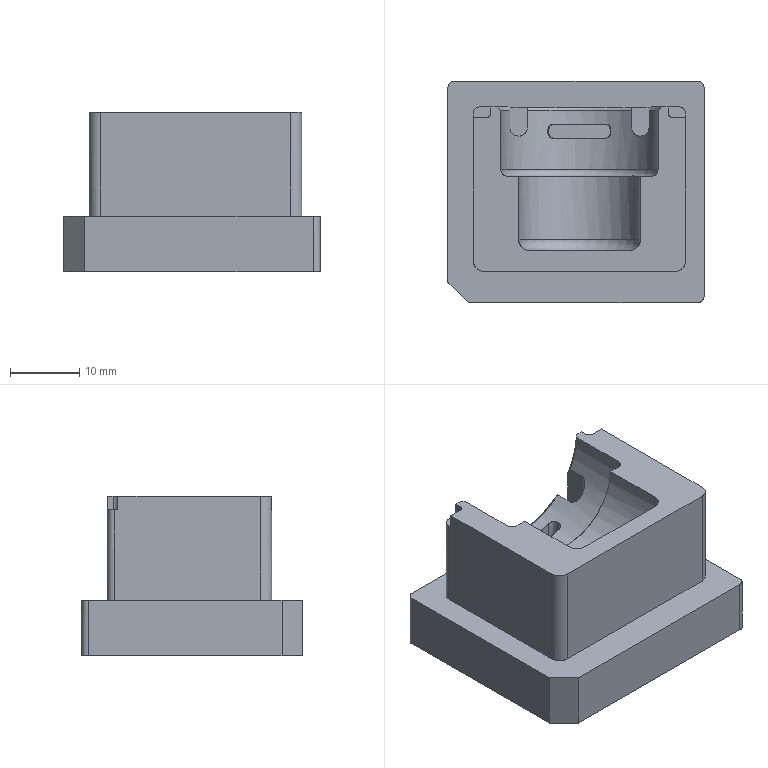NC program | PowerMill | posted with a generic post | part box 37 x 32 x 23 mm
Lines 26967 to 27634 of 159067:
N27064 M6
N27065 S8500 M03
N27066 G00 G90 X0.0 Y0.0
N27067 G43 Z11.8 H3
N27068
N27069 G05 P10000 R8
N27070 X-12.7401 Y22.8793
N27071 Z-1.156
N27072 G01 Z-2.356 F360.0
N27073 X-12.7403 Y17.6043 F600.0
N27074 X-12.8666 Y17.4744
N27075 G00 Z2.8538
N27076 G01 X-25.4619 Y11.9052 F10000.0
N27077 G00 Z-1.156
N27078 G01 Z-2.356 F360.0
N27079 X-20.1929 Y11.6533 F600.0
N27080 G03 X-19.9391 Y12.0208 I-0.3314 J0.5002
N27081 G01 X-19.8095 Y12.4495
N27082 X-19.6538 Y12.8389
N27083 X-19.4987 Y13.1574
N27084 X-19.3232 Y13.4633
N27085 X-19.2241 Y13.6177
N27086 X-18.9592 Y13.9792
N27087 X-18.6419 Y14.3407
N27088 X-18.5304 Y14.4536
N27089 X-18.134 Y14.804
N27090 X-17.7375 Y15.091
N27091 X-17.6051 Y15.1755
N27092 X-17.2749 Y15.3622
N27093 X-16.9447 Y15.5192
N27094 X-16.2702 Y15.7923
N27095 G03 X-16.0633 Y15.9321 I-0.2251 J0.5562
N27096 G01 X-15.7004 Y16.2688
N27097 X-15.359 Y16.5339
N27098 X-15.0563 Y16.7332
N27099 X-14.8146 Y16.8723
N27100 X-14.5661 Y16.9986
N27101 X-14.1697 Y17.1669
N27102 X-13.7733 Y17.299
N27103 X-13.3769 Y17.3969
N27104 X-12.9115 Y17.4687
N27105 G03 X-12.582 Y17.6043 I-0.0533 J0.5977
N27106 G00 Z2.8538
N27107 G01 X13.525 Y22.879 F10000.0
N27108 G00 Z-1.156
N27109 G01 Z-2.356 F360.0
N27110 X13.5779 Y17.6043 F600.0
N27111 G03 X13.9074 Y17.4687 I0.3828 J0.4621
N27112 G01 X14.3728 Y17.3969
N27113 X14.6204 Y17.3371
N27114 X14.8653 Y17.267
N27115 X15.1656 Y17.1669
N27116 X15.562 Y16.9986
N27117 X15.8105 Y16.8723
N27118 X16.0521 Y16.7332
N27119 X16.3549 Y16.5339
N27120 X16.6959 Y16.2694
N27121 X17.0591 Y15.9321
N27122 G03 X17.266 Y15.7923 I0.4321 J0.4164
N27123 G01 X17.9406 Y15.5192
N27124 X18.2704 Y15.3622
N27125 X18.601 Y15.1755
N27126 X18.7334 Y15.091
N27127 X19.1298 Y14.804
N27128 X19.5835 Y14.3966
N27129 X19.9014 Y14.0454
N27130 X20.22 Y13.6177
N27131 X20.3191 Y13.4633
N27132 X20.4947 Y13.1574
N27133 X20.6472 Y12.8453
N27134 X20.8047 Y12.4495
N27135 X20.9261 Y12.06
N27136 X21.0148 Y11.6706
N27137 X21.0771 Y11.219
N27138 G03 X21.2043 Y10.8918 I0.5983 J0.0443
N27139 G00 Z4.0
N27140 G01 X-24.9518 Y-13.4611 F10000.0
N27141 G00 Z0.8
N27142 G01 Z-0.4 F360.0
N27143 X-19.9022 Y-11.9356 F600.0
N27144 X20.9006 Y-11.9252
N27145 X21.042 Y-11.3912
N27146 X21.1226 Y-10.9631
N27147 X21.177 Y-10.5097
N27148 X21.2021 Y-10.0577
N27149 X21.2041 Y-7.0021
N27150 X-20.2078 Y-7.0126
N27151 X-20.208 Y-2.0896
N27152 X-2.9417 Y-2.0852
N27153 X-2.9457 Y2.3697
N27154 X-2.9685 Y2.7272
N27155 X-2.9834 Y2.8378
N27156 X-20.2082 Y2.8334
N27157 X-20.2084 Y7.7564
N27158 X-5.5055 Y7.7602
N27159 X-5.5061 Y11.8451
N27160 G03 X-5.589 Y12.6832 I-5.7385 J-0.1442
N27161 G01 X-19.8266 Y12.6796
N27162 G00 Z4.0
N27163 G01 X-1.3376 Y-2.083 F10000.0
N27164 G00 Z0.8
N27165 G01 Z-0.4 F360.0
N27166 X3.9374 Y-2.0835 F600.0
N27167 X21.204 Y-2.0791
N27168 X21.2038 Y2.8439
N27169 X3.9772 Y2.8395
N27170 G02 X4.2203 Y3.9177 I5.4024 J-0.6514
N27171 G01 X4.3607 Y4.2897
N27172 X4.5799 Y4.745
N27173 X4.6454 Y4.8536
N27174 G02 X5.1997 Y5.6551 I4.3119 J-2.3898
N27175 G01 X5.4158 Y5.8958
N27176 X5.7046 Y6.1763
N27177 X5.9771 Y6.4062
N27178 X6.2349 Y6.5958
N27179 X6.5011 Y6.7732
N27180 X6.5014 Y7.7632
N27181 X21.2037 Y7.7669
N27182 X21.2006 Y10.8927
N27183 G03 X21.0747 Y11.8712 I-5.6314 J-0.227
N27184 G03 X20.8204 Y12.6898 I-5.3043 J-1.199
N27185 G01 X6.5867 Y12.6862
N27186 G00 Z11.8
N27187 G05 P0
N27188 (---------------)
N27189 ( END TOOLPATH : 粗公基准台01-平坦面平行-D10 )
N27190 (---------------)
N27191 ( START TOOLPATH : 粗公基准台01-基准面偏置-D10 )
N27192 (---------------)
N27193 G00 X0.0 Y0.0 Z9.8
N27194 G05 P10000 R8
N27195 X-8.4072 Y-26.625
N27196 Z-14.0
N27197 G01 Z-15.2 F360.0
N27198 Y-21.35 F600.0
N27199 X0.7919 Y-16.7504
N27200 X-13.4626 Y-16.7466
N27201 X-13.8585 Y-16.7231
N27202 X-14.2545 Y-16.6774
N27203 X-15.0464 Y-16.5113
N27204 X-15.4424 Y-16.3928
N27205 X-15.8383 Y-16.2445
N27206 X-16.2343 Y-16.0695
N27207 X-16.6303 Y-15.8609
N27208 X-17.1233 Y-15.556
N27209 X-17.4222 Y-15.3388
N27210 X-17.8769 Y-14.959
N27211 X-18.2141 Y-14.6284
N27212 X-18.4232 Y-14.4
N27213 X-18.6258 Y-14.1528
N27214 X-18.8201 Y-13.8991
N27215 X-19.006 Y-13.6265
N27216 X-19.1529 Y-13.3844
N27217 X-19.372 Y-12.9907
N27218 X-19.5528 Y-12.597
N27219 X-19.6866 Y-12.2684
N27220 X-19.8366 Y-11.8097
N27221 X-19.9393 Y-11.4161
N27222 X-20.016 Y-11.0224
N27223 X-20.07 Y-10.6288
N27224 X-20.0988 Y-10.2351
N27225 X-20.1088 Y-9.4478
N27226 X-20.1061 Y11.4161
N27227 X-20.0825 Y11.8097
N27228 X-20.0454 Y12.1426
N27229 X-19.9627 Y12.597
N27230 X-19.7979 Y13.1998
N27231 X-19.7337 Y13.3844
N27232 X-19.5764 Y13.778
N27233 X-19.3857 Y14.1717
N27234 X-19.207 Y14.4858
N27235 X-19.006 Y14.7998
N27236 X-18.8923 Y14.959
N27237 X-18.578 Y15.348
N27238 X-18.2048 Y15.7463
N27239 X-17.8135 Y16.091
N27240 X-17.4222 Y16.3891
N27241 X-17.2041 Y16.5336
N27242 X-16.6303 Y16.8565
N27243 X-16.2343 Y17.0358
N27244 X-15.8383 Y17.1825
N27245 X-15.3573 Y17.3209
N27246 X-15.0464 Y17.3909
N27247 X-14.6505 Y17.454
N27248 X-14.2545 Y17.4901
N27249 X-13.5751 Y17.5049
N27250 X15.0464 Y17.5016
N27251 X15.4424 Y17.4753
N27252 X15.8383 Y17.427
N27253 X16.3534 Y17.3209
N27254 X16.6303 Y17.2471
N27255 X17.0262 Y17.115
N27256 X17.4222 Y16.9526
N27257 X17.8081 Y16.762
N27258 X18.2141 Y16.5252
N27259 X18.6101 Y16.2502
N27260 X19.006 Y15.9239
N27261 X19.2001 Y15.7463
N27262 X19.5204 Y15.4103
N27263 X19.8884 Y14.959
N27264 X20.1552 Y14.5653
N27265 X20.3818 Y14.1717
N27266 X20.5898 Y13.738
N27267 X20.7298 Y13.3844
N27268 X20.8314 Y13.0824
N27269 X20.9587 Y12.597
N27270 X21.0325 Y12.2034
N27271 X21.0778 Y11.8097
N27272 X21.1024 Y11.4161
N27273 X21.1049 Y-9.4478
N27274 X21.0941 Y-10.2351
N27275 X21.0657 Y-10.6288
N27276 X21.0121 Y-11.0224
N27277 X20.9352 Y-11.4161
N27278 X20.8319 Y-11.8097
N27279 X20.7228 Y-12.1549
N27280 X20.5481 Y-12.597
N27281 X20.3679 Y-12.9907
N27282 X20.149 Y-13.3844
N27283 X19.9842 Y-13.6542
N27284 X19.7979 Y-13.9241
N27285 X19.6069 Y-14.1717
N27286 X19.3279 Y-14.5027
N27287 X19.006 Y-14.8337
N27288 X18.873 Y-14.959
N27289 X18.5435 Y-15.2389
N27290 X18.2141 Y-15.4895
N27291 X17.8205 Y-15.7463
N27292 X17.4222 Y-15.9739
N27293 X17.0262 Y-16.1614
N27294 X16.6303 Y-16.3253
N27295 X15.9605 Y-16.5336
N27296 X15.4424 Y-16.6461
N27297 X15.0464 Y-16.7043
N27298 X14.2545 Y-16.7504
N27299 X0.7919
N27300 G00 Z9.8
N27301 G05 P0
N27302 (---------------)
N27303 ( END TOOLPATH : 粗公基准台01-基准面偏置-D10 )
N27304 (---------------)
N27305 ( START TOOLPATH : 粗公基准台01-外形侧光-D10 )
N27306 (---------------)
N27307 G00 X0.0 Y0.0 Z10.8
N27308 G05 P10000 R8
N27309 X19.6602 Y-14.3443
N27310 Z-13.97
N27311 G01 Z-15.17 F360.0
N27312 G03 X18.5771 Y-14.7249 I-0.0821 J-1.4977 F600.0
N27313 G02 X14.1984 Y-16.38 I-4.3278 J4.8298
N27314 G01 X-13.1666
N27315 G02 X-19.7384 Y-9.9389 I-0.0854 J6.486
N27316 G01 X-19.7386 Y11.2314
N27317 G02 X-13.9402 Y17.1338 I5.8849 J0.0182
N27318 G01 X0.5163 Y17.1342
N27319 X14.7151 Y17.1345
N27320 G02 X20.7344 Y11.2296 I0.1299 J-5.888
N27321 G01 X20.7343 Y-9.9404
N27322 G02 X19.792 Y-13.2619 I-6.485 J0.0453
N27323 G02 X18.5771 Y-14.7249 I-5.5426 J3.3668
N27324 G03 X18.0804 Y-15.7599 I1.001 J-1.1171
N27325 G01 X19.5989 Y-14.2944
N27326 G03 X18.5151 Y-14.6731 I-0.0848 J-1.4976
N27327 G02 X14.1984 Y-16.3 I-4.2656 J4.7779
N27328 G01 X-13.1658
N27329 G02 X-19.6584 Y-9.9389 I-0.0862 J6.406
N27330 G01 X-19.6586 Y11.2296
N27331 G02 X-13.9402 Y17.0538 I5.8049 J0.02
N27332 G01 X0.5163 Y17.0545
N27333 X14.7147
N27334 G02 X20.6544 Y11.2296 I0.1304 J-5.8079
N27335 G01 X20.6543 Y-9.9389
N27336 G02 X19.7236 Y-13.2204 I-6.4049 J0.0437
N27337 G02 X18.5151 Y-14.6731 I-5.4742 J3.3252
N27338 G03 X18.0165 Y-15.7072 I0.999 J-1.1189
N27339 G00 Z10.8
N27340 G05 P0
N27341 (---------------)
N27342 ( END TOOLPATH : 粗公基准台01-外形侧光-D10 )
N27343 (---------------)
N27344 ( START TOOLPATH : 粗公基准台01-基准台侧光-D10 )
N27345 (---------------)
N27346 G00 X0.0 Y0.0 Z9.8
N27347 G05 P10000 R8
N27348 X23.9377 Y-24.0084
N27349 Z-21.9
N27350 G01 Z-23.1 F360.0
N27351 G03 X20.9814 Y-19.976 I-1.4782 J2.0162 F600.0
N27352 G01 X20.8321 Y-20.0854
N27353 X20.8289 Y-20.0877
N27354 X20.8256 Y-20.0898
N27355 X20.3786 Y-20.3545
N27356 X20.3757 Y-20.3561
N27357 X20.3728 Y-20.3576
N27358 X19.9258 Y-20.5748
N27359 X19.9239 Y-20.5758
N27360 X19.9219 Y-20.5766
N27361 X19.783 Y-20.6351
N27362 X19.7814 Y-20.6357
N27363 X19.7798 Y-20.6363
N27364 X19.4717 Y-20.7508
N27365 X19.4692 Y-20.7517
N27366 X19.4667 Y-20.7525
N27367 X19.0197 Y-20.8857
N27368 X19.0169 Y-20.8864
N27369 X19.0141 Y-20.8871
N27370 X18.5671 Y-20.9854
N27371 X18.5639 Y-20.986
N27372 X18.5608 Y-20.9865
N27373 X18.1138 Y-21.0477
N27374 X18.111 Y-21.0481
N27375 X18.1081 Y-21.0483
N27376 X17.6611 Y-21.0774
N27377 X17.6588 Y-21.0775
N27378 X17.6564 Y-21.0776
N27379 X17.2094 Y-21.08
N27380 X17.2092
N27381 X17.2089
N27382 X-15.421
N27383 X-15.4222
N27384 X-15.4234
N27385 X-15.8704 Y-21.0664
N27386 X-15.8739 Y-21.0663
N27387 X-15.8775 Y-21.0659
N27388 X-16.3244 Y-21.0126
N27389 X-16.328 Y-21.0121
N27390 X-16.3316 Y-21.0114
N27391 X-16.7786 Y-20.9164
N27392 X-16.7822 Y-20.9156
N27393 X-16.7858 Y-20.9145
N27394 X-17.2327 Y-20.7753
N27395 X-17.2364 Y-20.774
N27396 X-17.2399 Y-20.7727
N27397 X-17.6869 Y-20.5851
N27398 X-17.6905 Y-20.5835
N27399 X-17.6941 Y-20.5817
N27400 X-18.141 Y-20.3394
N27401 X-18.1438 Y-20.3379
N27402 X-18.1465 Y-20.3362
N27403 X-18.3848 Y-20.1814
N27404 X-18.3866 Y-20.1802
N27405 X-18.3883 Y-20.179
N27406 X-18.5971 Y-20.0267
N27407 X-18.5993 Y-20.025
N27408 X-18.6015 Y-20.0232
N27409 X-18.9502 Y-19.7285
N27410 X-18.952 Y-19.7269
N27411 X-18.9538 Y-19.7253
N27412 X-19.052 Y-19.6317
N27413 X-19.0528 Y-19.6311
N27414 X-19.0535 Y-19.6304
N27415 X-22.0892 Y-16.595
N27416 X-22.0895 Y-16.5947
N27417 X-22.0899 Y-16.5943
N27418 X-22.1831 Y-16.4988
N27419 X-22.1847 Y-16.4971
N27420 X-22.1863 Y-16.4953
N27421 X-22.4902 Y-16.1438
N27422 X-22.4921 Y-16.1417
N27423 X-22.4938 Y-16.1394
N27424 X-22.6368 Y-15.9484
N27425 X-22.6381 Y-15.9466
N27426 X-22.6393 Y-15.9448
N27427 X-22.81 Y-15.6889
N27428 X-22.8118 Y-15.6861
N27429 X-22.8134 Y-15.6833
N27430 X-23.0612 Y-15.2363
N27431 X-23.063 Y-15.2328
N27432 X-23.0647 Y-15.2291
N27433 X-23.257 Y-14.7821
N27434 X-23.2585 Y-14.7786
N27435 X-23.2597 Y-14.775
N27436 X-23.4033 Y-14.328
N27437 X-23.4043 Y-14.3244
N27438 X-23.4052 Y-14.3208
N27439 X-23.5042 Y-13.8739
N27440 X-23.5049 Y-13.8703
N27441 X-23.5055 Y-13.8667
N27442 X-23.5626 Y-13.4197
N27443 X-23.563 Y-13.4161
N27444 X-23.5632 Y-13.4126
N27445 X-23.58 Y-12.9656
N27446 Y-12.9641
N27447 Y-12.9626
N27448 Y14.7505
N27449 Y14.7509
N27450 Y14.7512
N27451 X-23.5761 Y15.1982
N27452 X-23.576 Y15.2007
N27453 X-23.5759 Y15.2032
N27454 X-23.5442 Y15.6501
N27455 X-23.544 Y15.6531
N27456 X-23.5436 Y15.6559
N27457 X-23.479 Y16.1029
N27458 X-23.4785 Y16.1061
N27459 X-23.4778 Y16.1092
N27460 X-23.3765 Y16.5562
N27461 X-23.3758 Y16.5591
N27462 X-23.375 Y16.562
N27463 X-23.2375 Y17.009
N27464 X-23.2366 Y17.0116
N27465 X-23.2357 Y17.0142
N27466 X-23.0944 Y17.3807
N27467 X-23.0931 Y17.3839
N27468 X-23.0917 Y17.387
N27469 X-22.8346 Y17.9145
N27470 X-22.8329 Y17.9176
N27471 X-22.8312 Y17.9207
N27472 X-22.5621 Y18.3677
N27473 X-22.56 Y18.3709
N27474 X-22.5578 Y18.3741
N27475 X-22.2264 Y18.821
N27476 X-22.2242 Y18.8238
N27477 X-22.2219 Y18.8265
N27478 X-21.8246 Y19.2735
N27479 X-21.8228 Y19.2754
N27480 X-21.821 Y19.2773
N27481 X-21.735 Y19.3623
N27482 X-21.7334 Y19.3639
N27483 X-21.7316 Y19.3654
N27484 X-21.3199 Y19.7274
N27485 X-21.3172 Y19.7297
N27486 X-21.3144 Y19.7319
N27487 X-20.8321 Y20.0854
N27488 X-20.8289 Y20.0877
N27489 X-20.8256 Y20.0898
N27490 X-20.3786 Y20.3545
N27491 X-20.3757 Y20.3561
N27492 X-20.3728 Y20.3576
N27493 X-19.9258 Y20.5748
N27494 X-19.9228 Y20.5762
N27495 X-19.9197 Y20.5775
N27496 X-19.4727 Y20.7504
N27497 X-19.4698 Y20.7515
N27498 X-19.4667 Y20.7525
N27499 X-19.0197 Y20.8857
N27500 X-19.0169 Y20.8864
N27501 X-19.0141 Y20.8871
N27502 X-18.5671 Y20.9854
N27503 X-18.5639 Y20.986
N27504 X-18.5608 Y20.9865
N27505 X-18.1138 Y21.0477
N27506 X-18.111 Y21.0481
N27507 X-18.1081 Y21.0483
N27508 X-17.6611 Y21.0774
N27509 X-17.6588 Y21.0775
N27510 X-17.6564 Y21.0776
N27511 X-17.2094 Y21.08
N27512 X-17.2092
N27513 X-17.2089
N27514 X0.0
N27515 X17.2089
N27516 X17.2092
N27517 X17.2094
N27518 X17.6564 Y21.0776
N27519 X17.6588 Y21.0775
N27520 X17.6611 Y21.0774
N27521 X18.1081 Y21.0483
N27522 X18.111 Y21.0481
N27523 X18.1138 Y21.0477
N27524 X18.5608 Y20.9865
N27525 X18.5639 Y20.986
N27526 X18.5671 Y20.9854
N27527 X19.0141 Y20.8871
N27528 X19.0169 Y20.8864
N27529 X19.0197 Y20.8857
N27530 X19.4667 Y20.7525
N27531 X19.4698 Y20.7515
N27532 X19.4727 Y20.7504
N27533 X19.9197 Y20.5775
N27534 X19.9228 Y20.5762
N27535 X19.9258 Y20.5748
N27536 X20.3728 Y20.3576
N27537 X20.3757 Y20.3561
N27538 X20.3786 Y20.3545
N27539 X20.8256 Y20.0898
N27540 X20.8288 Y20.0878
N27541 X20.8318 Y20.0856
N27542 X21.2788 Y19.761
N27543 X21.2817 Y19.7588
N27544 X21.2845 Y19.7565
N27545 X21.7315 Y19.3656
N27546 X21.7333 Y19.3639
N27547 X21.735 Y19.3623
N27548 X21.821 Y19.2773
N27549 X21.8227 Y19.2755
N27550 X21.8244 Y19.2737
N27551 X22.1854 Y18.87
N27552 X22.1877 Y18.8674
N27553 X22.1898 Y18.8647
N27554 X22.5575 Y18.3744
N27555 X22.5599 Y18.3711
N27556 X22.5621 Y18.3677
N27557 X22.8312 Y17.9207
N27558 X22.8328 Y17.9179
N27559 X22.8343 Y17.915
N27560 X23.0561 Y17.468
N27561 X23.0575 Y17.4649
N27562 X23.0588 Y17.4618
N27563 X23.2355 Y17.0149
N27564 X23.2365 Y17.0119
N27565 X23.2375 Y17.009
N27566 X23.3749 Y16.562
N27567 X23.3758 Y16.5591
N27568 X23.3765 Y16.5562
N27569 X23.4778 Y16.1092
N27570 X23.4785 Y16.1061
N27571 X23.479 Y16.1029
N27572 X23.5436 Y15.6559
N27573 X23.544 Y15.6531
N27574 X23.5442 Y15.6502
N27575 X23.5759 Y15.2032
N27576 X23.5761 Y15.2007
N27577 Y15.1982
N27578 X23.58 Y14.7512
N27579 Y14.7509
N27580 Y14.7505
N27581 Y-14.7505
N27582 Y-14.7509
N27583 Y-14.7512
N27584 X23.5761 Y-15.1982
N27585 X23.576 Y-15.2007
N27586 X23.5759 Y-15.2032
N27587 X23.5442 Y-15.6501
N27588 X23.544 Y-15.6531
N27589 X23.5436 Y-15.6559
N27590 X23.479 Y-16.1029
N27591 X23.4785 Y-16.1061
N27592 X23.4778 Y-16.1092
N27593 X23.3765 Y-16.5562
N27594 X23.3758 Y-16.5591
N27595 X23.375 Y-16.562
N27596 X23.2375 Y-17.009
N27597 X23.2366 Y-17.0116
N27598 X23.2357 Y-17.0142
N27599 X23.0944 Y-17.3807
N27600 X23.0931 Y-17.3839
N27601 X23.0917 Y-17.387
N27602 X22.8346 Y-17.9145
N27603 X22.8329 Y-17.9176
N27604 X22.8312 Y-17.9207
N27605 X22.5621 Y-18.3677
N27606 X22.56 Y-18.3709
N27607 X22.5578 Y-18.3741
N27608 X22.2264 Y-18.821
N27609 X22.2242 Y-18.8238
N27610 X22.2219 Y-18.8265
N27611 X21.8246 Y-19.2735
N27612 X21.8228 Y-19.2754
N27613 X21.821 Y-19.2773
N27614 X21.735 Y-19.3623
N27615 X21.7334 Y-19.3639
N27616 X21.7316 Y-19.3654
N27617 X21.3199 Y-19.7274
N27618 X21.3172 Y-19.7297
N27619 X21.3144 Y-19.7319
N27620 X20.9814 Y-19.976
N27621 G03 X23.9377 Y-24.0084 I1.4782 J-2.0162
N27622 G01 X23.8863 Y-23.9469
N27623 G03 X20.9299 Y-19.9145 I-1.4782 J2.0162
N27624 G01 X20.7848 Y-20.0209
N27625 X20.3378 Y-20.2856
N27626 X19.8909 Y-20.5029
N27627 X19.7519 Y-20.5613
N27628 X19.4439 Y-20.6758
N27629 X18.9969 Y-20.809
N27630 X18.5499 Y-20.9072
N27631 X18.1029 Y-20.9685
N27632 X17.6559 Y-20.9976
N27633 X17.2089 Y-21.0
N27634 X-15.421
N27635 X-15.868 Y-20.9865
N27636 X-16.315 Y-20.9332
N27637 X-16.762 Y-20.8382
N27638 X-17.2089 Y-20.6989
N27639 X-17.6559 Y-20.5113
N27640 X-18.1029 Y-20.2691
N27641 X-18.3412 Y-20.1144
N27642 X-18.5499 Y-19.9621
N27643 X-18.8986 Y-19.6674
N27644 X-18.9969 Y-19.5738
N27645 X-22.0326 Y-16.5385
N27646 X-22.1258 Y-16.443
N27647 X-22.4297 Y-16.0915
N27648 X-22.5728 Y-15.9004
N27649 X-22.7435 Y-15.6445
N27650 X-22.9912 Y-15.1975
N27651 X-23.1836 Y-14.7505
N27652 X-23.3271 Y-14.3035
N27653 X-23.4261 Y-13.8566
N27654 X-23.4832 Y-13.4096
N27655 X-23.5 Y-12.9626
N27656 Y14.7505
N27657 X-23.4961 Y15.1975
N27658 X-23.4644 Y15.6445
N27659 X-23.3998 Y16.0915
N27660 X-23.2985 Y16.5385
N27661 X-23.161 Y16.9855
N27662 X-23.0198 Y17.352
N27663 X-22.7627 Y17.8794
N27664 X-22.4935 Y18.3264
N27665 X-22.1622 Y18.7734
N27666 X-21.7648 Y19.2204
N27667 X-21.6788 Y19.3053
N27668 X-21.2671 Y19.6674
N27669 X-20.7848 Y20.0209
N27670 X-20.3378 Y20.2856
N27671 X-19.8909 Y20.5029
N27672 X-19.4439 Y20.6758
N27673 X-18.9969 Y20.809
N27674 X-18.5499 Y20.9072
N27675 X-18.1029 Y20.9685
N27676 X-17.6559 Y20.9976
N27677 X-17.2089 Y21.0
N27678 X0.0
N27679 X17.2089
N27680 X17.6559 Y20.9976
N27681 X18.1029 Y20.9685
N27682 X18.5499 Y20.9072
N27683 X18.9969 Y20.809
N27684 X19.4439 Y20.6758
N27685 X19.8909 Y20.5029
N27686 X20.3378 Y20.2856
N27687 X20.7848 Y20.0209
N27688 X21.2318 Y19.6963
N27689 X21.6788 Y19.3053
N27690 X21.7648 Y19.2204
N27691 X22.1258 Y18.8167
N27692 X22.4935 Y18.3264
N27693 X22.7627 Y17.8794
N27694 X22.9844 Y17.4324
N27695 X23.1611 Y16.9855
N27696 X23.2985 Y16.5385
N27697 X23.3998 Y16.0915
N27698 X23.4644 Y15.6445
N27699 X23.4961 Y15.1975
N27700 X23.5 Y14.7505
N27701 Y-14.7505
N27702 X23.4961 Y-15.1975
N27703 X23.4644 Y-15.6445
N27704 X23.3998 Y-16.0915
N27705 X23.2985 Y-16.5385
N27706 X23.161 Y-16.9855
N27707 X23.0198 Y-17.352
N27708 X22.7627 Y-17.8794
N27709 X22.4935 Y-18.3264
N27710 X22.1622 Y-18.7734
N27711 X21.7648 Y-19.2204
N27712 X21.6788 Y-19.3053
N27713 X21.2671 Y-19.6674
N27714 X20.9299 Y-19.9145
N27715 G03 X23.8863 Y-23.9469 I1.4782 J-2.0162
N27716 G00 Z9.8
N27717 G05 P0
N27718 (---------------)
N27719 ( END TOOLPATH : 粗公基准台01-基准台侧光-D10 )
N27720 (---------------)
N27721
N27722 M05
N27723 G53 Z0.0
N27724 (---------------)
N27725 ( START TOOLPATH : 粗公精光01-最佳等高-R1.5 )
N27726 (---------------)
N27727 ( TOOL NO.    :22 )
N27728 ( TOOL TYPE   : BALLNOSED)
N27729 ( TOOL ID     : R1.5_2_1)
N27730 ( TOOL DIA    : 3.0 LENGTH 67.36)
N27731 T22